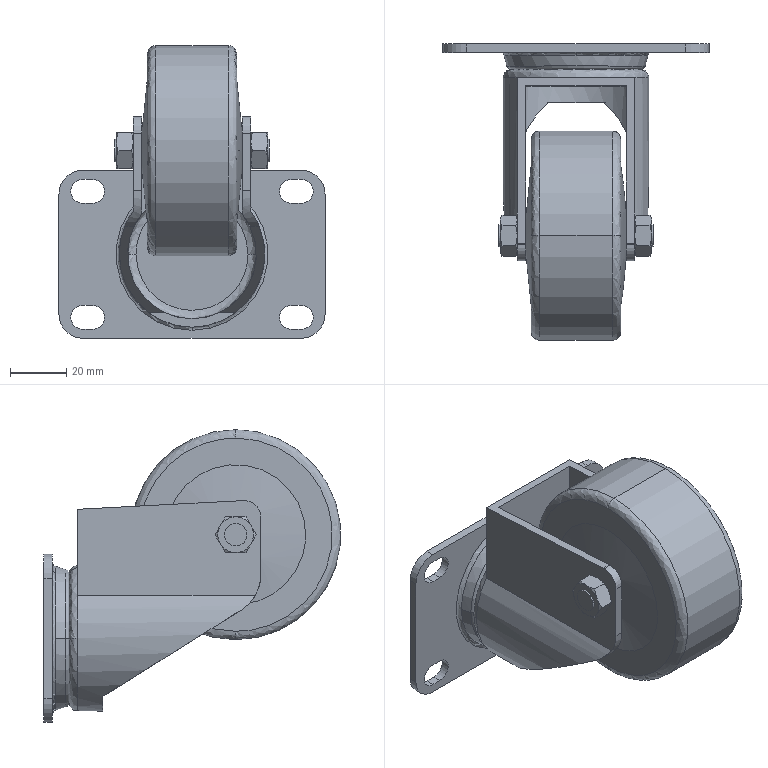Part | SolidWorks | features ICE 4, BaseBody 2, Fillet 2, Extrusion 1, Revolution 1 | 3 solids | 130 faces | box 95 x 106 x 104.5 mm | volume 205443 mm3 | plane 51 | cylinder 38 | cone 26 | spline 11 | torus 4 | commonest cylinder face diameters 8.5 x12 8 x8 12 x4 12.75 x4 17 x4 30 x2